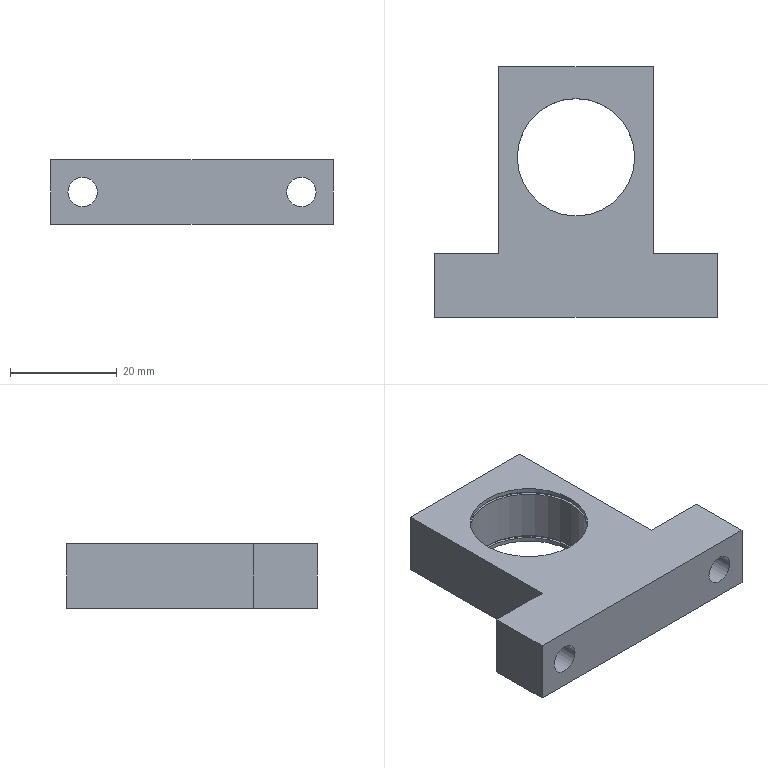Part | SolidWorks | features ICE 4, Extrusion 1 | 1 solid | 34 faces | box 53 x 47 x 12 mm | volume 14009 mm3 | cylinder 18 | plane 16 | commonest cylinder face diameters 22 x6 5.5 x4 10 x4 23 x4
STEP:
#1=CARTESIAN_POINT('',(21.73,13.962,1.25));
#2=VERTEX_POINT('',#1);
#3=CARTESIAN_POINT('',(-1.27,13.962,1.25));
#4=VERTEX_POINT('',#3);
#5=CARTESIAN_POINT('',(10.23,13.962,1.25));
#6=DIRECTION('',(0.,0.,-1.));
#7=DIRECTION('',(-1.,0.,0.));
#8=AXIS2_PLACEMENT_3D('',#5,#6,#7);
#9=CIRCLE('',#8,11.5);
#10=EDGE_CURVE('',#2,#4,#9,.T.);
#11=ORIENTED_EDGE('',*,*,#10,.F.);
#12=CARTESIAN_POINT('',(21.73,13.962,0.75));
#13=VERTEX_POINT('',#12);
#14=CARTESIAN_POINT('',(21.73,13.962,1.25));
#15=DIRECTION('',(0.,0.,-1.));
#16=VECTOR('',#15,1000.);
#17=LINE('',#14,#16);
#18=EDGE_CURVE('',#2,#13,#17,.T.);
#19=ORIENTED_EDGE('',*,*,#18,.T.);
#20=CARTESIAN_POINT('',(-1.27,13.962,0.75));
#21=VERTEX_POINT('',#20);
#22=CARTESIAN_POINT('',(10.23,13.962,0.75));
#23=DIRECTION('',(0.,0.,-1.));
#24=DIRECTION('',(-1.,0.,0.));
#25=AXIS2_PLACEMENT_3D('',#22,#23,#24);
#26=CIRCLE('',#25,11.5);
#27=EDGE_CURVE('',#13,#21,#26,.T.);
#28=ORIENTED_EDGE('',*,*,#27,.T.);
#29=CARTESIAN_POINT('',(-1.27,13.962,1.25));
#30=DIRECTION('',(0.,0.,-1.));
#31=VECTOR('',#30,1000.);
#32=LINE('',#29,#31);
#33=EDGE_CURVE('',#4,#21,#32,.T.);
#34=ORIENTED_EDGE('',*,*,#33,.F.);
#35=EDGE_LOOP('',(#11,#19,#28,#34));
#36=FACE_OUTER_BOUND('',#35,.T.);
#37=CARTESIAN_POINT('',(10.23,13.962,1.25));
#38=DIRECTION('',(0.,0.,-1.));
#39=DIRECTION('',(-1.,0.,0.));
#40=AXIS2_PLACEMENT_3D('',#37,#38,#39);
#41=CYLINDRICAL_SURFACE('',#40,11.5);
#42=ADVANCED_FACE('',(#36),#41,.F.);
#43=CARTESIAN_POINT('',(-1.27,13.962,10.75));
#44=VERTEX_POINT('',#43);
#45=CARTESIAN_POINT('',(21.73,13.962,10.75));
#46=VERTEX_POINT('',#45);
#47=CARTESIAN_POINT('',(10.23,13.962,10.75));
#48=DIRECTION('',(0.,0.,1.));
#49=DIRECTION('',(1.,0.,0.));
#50=AXIS2_PLACEMENT_3D('',#47,#48,#49);
#51=CIRCLE('',#50,11.5);
#52=EDGE_CURVE('',#44,#46,#51,.T.);
#53=ORIENTED_EDGE('',*,*,#52,.F.);
#54=CARTESIAN_POINT('',(-1.27,13.962,11.25));
#55=VERTEX_POINT('',#54);
#56=CARTESIAN_POINT('',(-1.27,13.962,10.75));
#57=DIRECTION('',(0.,0.,1.));
#58=VECTOR('',#57,1000.);
#59=LINE('',#56,#58);
#60=EDGE_CURVE('',#44,#55,#59,.T.);
#61=ORIENTED_EDGE('',*,*,#60,.T.);
#62=CARTESIAN_POINT('',(21.73,13.962,11.25));
#63=VERTEX_POINT('',#62);
#64=CARTESIAN_POINT('',(10.23,13.962,11.25));
#65=DIRECTION('',(0.,0.,1.));
#66=DIRECTION('',(1.,0.,0.));
#67=AXIS2_PLACEMENT_3D('',#64,#65,#66);
#68=CIRCLE('',#67,11.5);
#69=EDGE_CURVE('',#55,#63,#68,.T.);
#70=ORIENTED_EDGE('',*,*,#69,.T.);
#71=CARTESIAN_POINT('',(21.73,13.962,10.75));
#72=DIRECTION('',(0.,0.,1.));
#73=VECTOR('',#72,1000.);
#74=LINE('',#71,#73);
#75=EDGE_CURVE('',#46,#63,#74,.T.);
#76=ORIENTED_EDGE('',*,*,#75,.F.);
#77=EDGE_LOOP('',(#53,#61,#70,#76));
#78=FACE_OUTER_BOUND('',#77,.T.);
#79=CARTESIAN_POINT('',(10.23,13.962,10.75));
#80=DIRECTION('',(0.,0.,1.));
#81=DIRECTION('',(1.,0.,0.));
#82=AXIS2_PLACEMENT_3D('',#79,#80,#81);
#83=CYLINDRICAL_SURFACE('',#82,11.5);
#84=ADVANCED_FACE('',(#78),#83,.F.);
#85=CARTESIAN_POINT('',(-5.27,-9.838,6.));
#86=VERTEX_POINT('',#85);
#87=CARTESIAN_POINT('',(-15.27,-9.838,6.));
#88=VERTEX_POINT('',#87);
#89=CARTESIAN_POINT('',(-10.27,-9.838,6.));
#90=DIRECTION('',(0.,1.,0.));
#91=DIRECTION('',(-1.,0.,0.));
#92=AXIS2_PLACEMENT_3D('',#89,#90,#91);
#93=CIRCLE('',#92,5.);
#94=EDGE_CURVE('',#86,#88,#93,.T.);
#95=ORIENTED_EDGE('',*,*,#94,.F.);
#96=CARTESIAN_POINT('',(-5.27,-4.038,6.));
#97=VERTEX_POINT('',#96);
#98=CARTESIAN_POINT('',(-5.27,-9.838,6.));
#99=DIRECTION('',(0.,1.,0.));
#100=VECTOR('',#99,1000.);
#101=LINE('',#98,#100);
#102=EDGE_CURVE('',#86,#97,#101,.T.);
#103=ORIENTED_EDGE('',*,*,#102,.T.);
#104=CARTESIAN_POINT('',(-15.27,-4.038,6.));
#105=VERTEX_POINT('',#104);
#106=CARTESIAN_POINT('',(-10.27,-4.038,6.));
#107=DIRECTION('',(0.,1.,0.));
#108=DIRECTION('',(-1.,0.,0.));
#109=AXIS2_PLACEMENT_3D('',#106,#107,#108);
#110=CIRCLE('',#109,5.);
#111=EDGE_CURVE('',#97,#105,#110,.T.);
#112=ORIENTED_EDGE('',*,*,#111,.T.);
#113=CARTESIAN_POINT('',(-15.27,-9.838,6.));
#114=DIRECTION('',(0.,1.,0.));
#115=VECTOR('',#114,1000.);
#116=LINE('',#113,#115);
#117=EDGE_CURVE('',#88,#105,#116,.T.);
#118=ORIENTED_EDGE('',*,*,#117,.F.);
#119=EDGE_LOOP('',(#95,#103,#112,#118));
#120=FACE_OUTER_BOUND('',#119,.T.);
#121=CARTESIAN_POINT('',(-10.27,-9.838,6.));
#122=DIRECTION('',(0.,1.,0.));
#123=DIRECTION('',(-1.,0.,0.));
#124=AXIS2_PLACEMENT_3D('',#121,#122,#123);
#125=CYLINDRICAL_SURFACE('',#124,5.);
#126=ADVANCED_FACE('',(#120),#125,.F.);
#127=CARTESIAN_POINT('',(35.73,-9.838,6.));
#128=VERTEX_POINT('',#127);
#129=CARTESIAN_POINT('',(25.73,-9.838,6.));
#130=VERTEX_POINT('',#129);
#131=CARTESIAN_POINT('',(30.73,-9.838,6.));
#132=DIRECTION('',(0.,1.,0.));
#133=DIRECTION('',(-1.,0.,0.));
#134=AXIS2_PLACEMENT_3D('',#131,#132,#133);
#135=CIRCLE('',#134,5.);
#136=EDGE_CURVE('',#128,#130,#135,.T.);
#137=ORIENTED_EDGE('',*,*,#136,.F.);
#138=CARTESIAN_POINT('',(35.73,-4.038,6.));
#139=VERTEX_POINT('',#138);
#140=CARTESIAN_POINT('',(35.73,-9.838,6.));
#141=DIRECTION('',(0.,1.,0.));
#142=VECTOR('',#141,1000.);
#143=LINE('',#140,#142);
#144=EDGE_CURVE('',#128,#139,#143,.T.);
#145=ORIENTED_EDGE('',*,*,#144,.T.);
#146=CARTESIAN_POINT('',(25.73,-4.038,6.));
#147=VERTEX_POINT('',#146);
#148=CARTESIAN_POINT('',(30.73,-4.038,6.));
#149=DIRECTION('',(0.,1.,0.));
#150=DIRECTION('',(-1.,0.,0.));
#151=AXIS2_PLACEMENT_3D('',#148,#149,#150);
#152=CIRCLE('',#151,5.);
#153=EDGE_CURVE('',#139,#147,#152,.T.);
#154=ORIENTED_EDGE('',*,*,#153,.T.);
#155=CARTESIAN_POINT('',(25.73,-9.838,6.));
#156=DIRECTION('',(0.,1.,0.));
#157=VECTOR('',#156,1000.);
#158=LINE('',#155,#157);
#159=EDGE_CURVE('',#130,#147,#158,.T.);
#160=ORIENTED_EDGE('',*,*,#159,.F.);
#161=EDGE_LOOP('',(#137,#145,#154,#160));
#162=FACE_OUTER_BOUND('',#161,.T.);
#163=CARTESIAN_POINT('',(30.73,-9.838,6.));
#164=DIRECTION('',(0.,1.,0.));
#165=DIRECTION('',(-1.,0.,0.));
#166=AXIS2_PLACEMENT_3D('',#163,#164,#165);
#167=CYLINDRICAL_SURFACE('',#166,5.);
#168=ADVANCED_FACE('',(#162),#167,.F.);
#169=CARTESIAN_POINT('',(-0.7697,13.962,12.));
#170=VERTEX_POINT('',#169);
#171=CARTESIAN_POINT('',(21.23,13.962,12.));
#172=VERTEX_POINT('',#171);
#173=CARTESIAN_POINT('',(10.23,13.962,12.));
#174=DIRECTION('',(0.,0.,1.));
#175=DIRECTION('',(1.,0.,0.));
#176=AXIS2_PLACEMENT_3D('',#173,#174,#175);
#177=CIRCLE('',#176,11.);
#178=EDGE_CURVE('',#170,#172,#177,.T.);
#179=ORIENTED_EDGE('',*,*,#178,.T.);
#180=CARTESIAN_POINT('',(21.23,13.962,11.25));
#181=VERTEX_POINT('',#180);
#182=CARTESIAN_POINT('',(21.23,13.962,12.));
#183=DIRECTION('',(0.,0.,-1.));
#184=VECTOR('',#183,1000.);
#185=LINE('',#182,#184);
#186=EDGE_CURVE('',#172,#181,#185,.T.);
#187=ORIENTED_EDGE('',*,*,#186,.T.);
#188=CARTESIAN_POINT('',(-0.7697,13.962,11.25));
#189=VERTEX_POINT('',#188);
#190=CARTESIAN_POINT('',(10.23,13.962,11.25));
#191=DIRECTION('',(0.,0.,1.));
#192=DIRECTION('',(1.,0.,0.));
#193=AXIS2_PLACEMENT_3D('',#190,#191,#192);
#194=CIRCLE('',#193,11.);
#195=EDGE_CURVE('',#189,#181,#194,.T.);
#196=ORIENTED_EDGE('',*,*,#195,.F.);
#197=CARTESIAN_POINT('',(-0.7697,13.962,12.));
#198=DIRECTION('',(0.,0.,-1.));
#199=VECTOR('',#198,1000.);
#200=LINE('',#197,#199);
#201=EDGE_CURVE('',#170,#189,#200,.T.);
#202=ORIENTED_EDGE('',*,*,#201,.F.);
#203=EDGE_LOOP('',(#179,#187,#196,#202));
#204=FACE_OUTER_BOUND('',#203,.T.);
#205=CARTESIAN_POINT('',(10.23,13.962,12.));
#206=DIRECTION('',(0.,0.,-1.));
#207=DIRECTION('',(-1.,0.,0.));
#208=AXIS2_PLACEMENT_3D('',#205,#206,#207);
#209=CYLINDRICAL_SURFACE('',#208,11.);
#210=ADVANCED_FACE('',(#204),#209,.F.);
#211=CARTESIAN_POINT('',(33.48,-16.038,6.));
#212=VERTEX_POINT('',#211);
#213=CARTESIAN_POINT('',(27.98,-16.038,6.));
#214=VERTEX_POINT('',#213);
#215=CARTESIAN_POINT('',(30.73,-16.038,6.));
#216=DIRECTION('',(0.,1.,0.));
#217=DIRECTION('',(-1.,0.,0.));
#218=AXIS2_PLACEMENT_3D('',#215,#216,#217);
#219=CIRCLE('',#218,2.75);
#220=EDGE_CURVE('',#212,#214,#219,.T.);
#221=ORIENTED_EDGE('',*,*,#220,.F.);
#222=CARTESIAN_POINT('',(33.48,-9.838,6.));
#223=VERTEX_POINT('',#222);
#224=CARTESIAN_POINT('',(33.48,-16.038,6.));
#225=DIRECTION('',(0.,1.,0.));
#226=VECTOR('',#225,1000.);
#227=LINE('',#224,#226);
#228=EDGE_CURVE('',#212,#223,#227,.T.);
#229=ORIENTED_EDGE('',*,*,#228,.T.);
#230=CARTESIAN_POINT('',(27.98,-9.838,6.));
#231=VERTEX_POINT('',#230);
#232=CARTESIAN_POINT('',(30.73,-9.838,6.));
#233=DIRECTION('',(0.,-1.,0.));
#234=DIRECTION('',(-1.,0.,0.));
#235=AXIS2_PLACEMENT_3D('',#232,#233,#234);
#236=CIRCLE('',#235,2.75);
#237=EDGE_CURVE('',#231,#223,#236,.T.);
#238=ORIENTED_EDGE('',*,*,#237,.F.);
#239=CARTESIAN_POINT('',(27.98,-16.038,6.));
#240=DIRECTION('',(0.,1.,0.));
#241=VECTOR('',#240,1000.);
#242=LINE('',#239,#241);
#243=EDGE_CURVE('',#214,#231,#242,.T.);
#244=ORIENTED_EDGE('',*,*,#243,.F.);
#245=EDGE_LOOP('',(#221,#229,#238,#244));
#246=FACE_OUTER_BOUND('',#245,.T.);
#247=CARTESIAN_POINT('',(30.73,-16.038,6.));
#248=DIRECTION('',(0.,1.,0.));
#249=DIRECTION('',(-1.,0.,0.));
#250=AXIS2_PLACEMENT_3D('',#247,#248,#249);
#251=CYLINDRICAL_SURFACE('',#250,2.75);
#252=ADVANCED_FACE('',(#246),#251,.F.);
#253=CARTESIAN_POINT('',(-7.52,-16.038,6.));
#254=VERTEX_POINT('',#253);
#255=CARTESIAN_POINT('',(-13.02,-16.038,6.));
#256=VERTEX_POINT('',#255);
#257=CARTESIAN_POINT('',(-10.27,-16.038,6.));
#258=DIRECTION('',(0.,1.,0.));
#259=DIRECTION('',(-1.,0.,0.));
#260=AXIS2_PLACEMENT_3D('',#257,#258,#259);
#261=CIRCLE('',#260,2.75);
#262=EDGE_CURVE('',#254,#256,#261,.T.);
#263=ORIENTED_EDGE('',*,*,#262,.F.);
#264=CARTESIAN_POINT('',(-7.52,-9.838,6.));
#265=VERTEX_POINT('',#264);
#266=CARTESIAN_POINT('',(-7.52,-16.038,6.));
#267=DIRECTION('',(0.,1.,0.));
#268=VECTOR('',#267,1000.);
#269=LINE('',#266,#268);
#270=EDGE_CURVE('',#254,#265,#269,.T.);
#271=ORIENTED_EDGE('',*,*,#270,.T.);
#272=CARTESIAN_POINT('',(-13.02,-9.838,6.));
#273=VERTEX_POINT('',#272);
#274=CARTESIAN_POINT('',(-10.27,-9.838,6.));
#275=DIRECTION('',(0.,-1.,0.));
#276=DIRECTION('',(-1.,0.,0.));
#277=AXIS2_PLACEMENT_3D('',#274,#275,#276);
#278=CIRCLE('',#277,2.75);
#279=EDGE_CURVE('',#273,#265,#278,.T.);
#280=ORIENTED_EDGE('',*,*,#279,.F.);
#281=CARTESIAN_POINT('',(-13.02,-16.038,6.));
#282=DIRECTION('',(0.,1.,0.));
#283=VECTOR('',#282,1000.);
#284=LINE('',#281,#283);
#285=EDGE_CURVE('',#256,#273,#284,.T.);
#286=ORIENTED_EDGE('',*,*,#285,.F.);
#287=EDGE_LOOP('',(#263,#271,#280,#286));
#288=FACE_OUTER_BOUND('',#287,.T.);
#289=CARTESIAN_POINT('',(-10.27,-16.038,6.));
#290=DIRECTION('',(0.,1.,0.));
#291=DIRECTION('',(-1.,0.,0.));
#292=AXIS2_PLACEMENT_3D('',#289,#290,#291);
#293=CYLINDRICAL_SURFACE('',#292,2.75);
#294=ADVANCED_FACE('',(#288),#293,.F.);
#295=CARTESIAN_POINT('',(21.23,13.962,0.75));
#296=VERTEX_POINT('',#295);
#297=CARTESIAN_POINT('',(-0.7697,13.962,0.75));
#298=VERTEX_POINT('',#297);
#299=CARTESIAN_POINT('',(10.23,13.962,0.75));
#300=DIRECTION('',(0.,0.,-1.));
#301=DIRECTION('',(-1.,0.,0.));
#302=AXIS2_PLACEMENT_3D('',#299,#300,#301);
#303=CIRCLE('',#302,11.);
#304=EDGE_CURVE('',#296,#298,#303,.T.);
#305=ORIENTED_EDGE('',*,*,#304,.F.);
#306=CARTESIAN_POINT('',(21.23,13.962,0.));
#307=VERTEX_POINT('',#306);
#308=CARTESIAN_POINT('',(21.23,13.962,12.));
#309=DIRECTION('',(0.,0.,-1.));
#310=VECTOR('',#309,1000.);
#311=LINE('',#308,#310);
#312=EDGE_CURVE('',#296,#307,#311,.T.);
#313=ORIENTED_EDGE('',*,*,#312,.T.);
#314=CARTESIAN_POINT('',(-0.7697,13.962,0.));
#315=VERTEX_POINT('',#314);
#316=CARTESIAN_POINT('',(10.23,13.962,0.));
#317=DIRECTION('',(0.,0.,1.));
#318=DIRECTION('',(1.,0.,0.));
#319=AXIS2_PLACEMENT_3D('',#316,#317,#318);
#320=CIRCLE('',#319,11.);
#321=EDGE_CURVE('',#315,#307,#320,.T.);
#322=ORIENTED_EDGE('',*,*,#321,.F.);
#323=CARTESIAN_POINT('',(-0.7697,13.962,12.));
#324=DIRECTION('',(0.,0.,-1.));
#325=VECTOR('',#324,1000.);
#326=LINE('',#323,#325);
#327=EDGE_CURVE('',#298,#315,#326,.T.);
#328=ORIENTED_EDGE('',*,*,#327,.F.);
#329=EDGE_LOOP('',(#305,#313,#322,#328));
#330=FACE_OUTER_BOUND('',#329,.T.);
#331=CARTESIAN_POINT('',(10.23,13.962,12.));
#332=DIRECTION('',(0.,0.,-1.));
#333=DIRECTION('',(-1.,0.,0.));
#334=AXIS2_PLACEMENT_3D('',#331,#332,#333);
#335=CYLINDRICAL_SURFACE('',#334,11.);
#336=ADVANCED_FACE('',(#330),#335,.F.);
#337=CARTESIAN_POINT('',(-0.7697,13.962,10.75));
#338=VERTEX_POINT('',#337);
#339=CARTESIAN_POINT('',(21.23,13.962,10.75));
#340=VERTEX_POINT('',#339);
#341=CARTESIAN_POINT('',(10.23,13.962,10.75));
#342=DIRECTION('',(0.,0.,1.));
#343=DIRECTION('',(1.,0.,0.));
#344=AXIS2_PLACEMENT_3D('',#341,#342,#343);
#345=CIRCLE('',#344,11.);
#346=EDGE_CURVE('',#338,#340,#345,.T.);
#347=ORIENTED_EDGE('',*,*,#346,.T.);
#348=CARTESIAN_POINT('',(21.23,13.962,1.25));
#349=VERTEX_POINT('',#348);
#350=CARTESIAN_POINT('',(21.23,13.962,12.));
#351=DIRECTION('',(0.,0.,-1.));
#352=VECTOR('',#351,1000.);
#353=LINE('',#350,#352);
#354=EDGE_CURVE('',#340,#349,#353,.T.);
#355=ORIENTED_EDGE('',*,*,#354,.T.);
#356=CARTESIAN_POINT('',(-0.7697,13.962,1.25));
#357=VERTEX_POINT('',#356);
#358=CARTESIAN_POINT('',(10.23,13.962,1.25));
#359=DIRECTION('',(0.,0.,-1.));
#360=DIRECTION('',(-1.,0.,0.));
#361=AXIS2_PLACEMENT_3D('',#358,#359,#360);
#362=CIRCLE('',#361,11.);
#363=EDGE_CURVE('',#349,#357,#362,.T.);
#364=ORIENTED_EDGE('',*,*,#363,.T.);
#365=CARTESIAN_POINT('',(-0.7697,13.962,12.));
#366=DIRECTION('',(0.,0.,-1.));
#367=VECTOR('',#366,1000.);
#368=LINE('',#365,#367);
#369=EDGE_CURVE('',#338,#357,#368,.T.);
#370=ORIENTED_EDGE('',*,*,#369,.F.);
#371=EDGE_LOOP('',(#347,#355,#364,#370));
#372=FACE_OUTER_BOUND('',#371,.T.);
#373=CARTESIAN_POINT('',(10.23,13.962,12.));
#374=DIRECTION('',(0.,0.,-1.));
#375=DIRECTION('',(-1.,0.,0.));
#376=AXIS2_PLACEMENT_3D('',#373,#374,#375);
#377=CYLINDRICAL_SURFACE('',#376,11.);
#378=ADVANCED_FACE('',(#372),#377,.F.);
#379=ORIENTED_EDGE('',*,*,#354,.F.);
#380=CARTESIAN_POINT('',(10.23,13.962,10.75));
#381=DIRECTION('',(0.,0.,1.));
#382=DIRECTION('',(1.,0.,0.));
#383=AXIS2_PLACEMENT_3D('',#380,#381,#382);
#384=CIRCLE('',#383,11.);
#385=EDGE_CURVE('',#340,#338,#384,.T.);
#386=ORIENTED_EDGE('',*,*,#385,.T.);
#387=ORIENTED_EDGE('',*,*,#369,.T.);
#388=CARTESIAN_POINT('',(10.23,13.962,1.25));
#389=DIRECTION('',(0.,0.,-1.));
#390=DIRECTION('',(-1.,0.,0.));
#391=AXIS2_PLACEMENT_3D('',#388,#389,#390);
#392=CIRCLE('',#391,11.);
#393=EDGE_CURVE('',#357,#349,#392,.T.);
#394=ORIENTED_EDGE('',*,*,#393,.T.);
#395=EDGE_LOOP('',(#379,#386,#387,#394));
#396=FACE_OUTER_BOUND('',#395,.T.);
#397=CARTESIAN_POINT('',(10.23,13.962,12.));
#398=DIRECTION('',(0.,0.,-1.));
#399=DIRECTION('',(-1.,0.,0.));
#400=AXIS2_PLACEMENT_3D('',#397,#398,#399);
#401=CYLINDRICAL_SURFACE('',#400,11.);
#402=ADVANCED_FACE('',(#396),#401,.F.);
#403=ORIENTED_EDGE('',*,*,#312,.F.);
#404=CARTESIAN_POINT('',(10.23,13.962,0.75));
#405=DIRECTION('',(0.,0.,-1.));
#406=DIRECTION('',(-1.,0.,0.));
#407=AXIS2_PLACEMENT_3D('',#404,#405,#406);
#408=CIRCLE('',#407,11.);
#409=EDGE_CURVE('',#298,#296,#408,.T.);
#410=ORIENTED_EDGE('',*,*,#409,.F.);
#411=ORIENTED_EDGE('',*,*,#327,.T.);
#412=CARTESIAN_POINT('',(10.23,13.962,0.));
#413=DIRECTION('',(0.,0.,1.));
#414=DIRECTION('',(1.,0.,0.));
#415=AXIS2_PLACEMENT_3D('',#412,#413,#414);
#416=CIRCLE('',#415,11.);
#417=EDGE_CURVE('',#307,#315,#416,.T.);
#418=ORIENTED_EDGE('',*,*,#417,.F.);
#419=EDGE_LOOP('',(#403,#410,#411,#418));
#420=FACE_OUTER_BOUND('',#419,.T.);
#421=CARTESIAN_POINT('',(10.23,13.962,12.));
#422=DIRECTION('',(0.,0.,-1.));
#423=DIRECTION('',(-1.,0.,0.));
#424=AXIS2_PLACEMENT_3D('',#421,#422,#423);
#425=CYLINDRICAL_SURFACE('',#424,11.);
#426=ADVANCED_FACE('',(#420),#425,.F.);
#427=ORIENTED_EDGE('',*,*,#270,.F.);
#428=CARTESIAN_POINT('',(-10.27,-16.038,6.));
#429=DIRECTION('',(0.,1.,0.));
#430=DIRECTION('',(-1.,0.,0.));
#431=AXIS2_PLACEMENT_3D('',#428,#429,#430);
#432=CIRCLE('',#431,2.75);
#433=EDGE_CURVE('',#256,#254,#432,.T.);
#434=ORIENTED_EDGE('',*,*,#433,.F.);
#435=ORIENTED_EDGE('',*,*,#285,.T.);
#436=CARTESIAN_POINT('',(-10.27,-9.838,6.));
#437=DIRECTION('',(0.,-1.,0.));
#438=DIRECTION('',(-1.,0.,0.));
#439=AXIS2_PLACEMENT_3D('',#436,#437,#438);
#440=CIRCLE('',#439,2.75);
#441=EDGE_CURVE('',#265,#273,#440,.T.);
#442=ORIENTED_EDGE('',*,*,#441,.F.);
#443=EDGE_LOOP('',(#427,#434,#435,#442));
#444=FACE_OUTER_BOUND('',#443,.T.);
#445=CARTESIAN_POINT('',(-10.27,-16.038,6.));
#446=DIRECTION('',(0.,1.,0.));
#447=DIRECTION('',(-1.,0.,0.));
#448=AXIS2_PLACEMENT_3D('',#445,#446,#447);
#449=CYLINDRICAL_SURFACE('',#448,2.75);
#450=ADVANCED_FACE('',(#444),#449,.F.);
#451=ORIENTED_EDGE('',*,*,#228,.F.);
#452=CARTESIAN_POINT('',(30.73,-16.038,6.));
#453=DIRECTION('',(0.,1.,0.));
#454=DIRECTION('',(-1.,0.,0.));
#455=AXIS2_PLACEMENT_3D('',#452,#453,#454);
#456=CIRCLE('',#455,2.75);
#457=EDGE_CURVE('',#214,#212,#456,.T.);
#458=ORIENTED_EDGE('',*,*,#457,.F.);
#459=ORIENTED_EDGE('',*,*,#243,.T.);
#460=CARTESIAN_POINT('',(30.73,-9.838,6.));
#461=DIRECTION('',(0.,-1.,0.));
#462=DIRECTION('',(-1.,0.,0.));
#463=AXIS2_PLACEMENT_3D('',#460,#461,#462);
#464=CIRCLE('',#463,2.75);
#465=EDGE_CURVE('',#223,#231,#464,.T.);
#466=ORIENTED_EDGE('',*,*,#465,.F.);
#467=EDGE_LOOP('',(#451,#458,#459,#466));
#468=FACE_OUTER_BOUND('',#467,.T.);
#469=CARTESIAN_POINT('',(30.73,-16.038,6.));
#470=DIRECTION('',(0.,1.,0.));
#471=DIRECTION('',(-1.,0.,0.));
#472=AXIS2_PLACEMENT_3D('',#469,#470,#471);
#473=CYLINDRICAL_SURFACE('',#472,2.75);
#474=ADVANCED_FACE('',(#468),#473,.F.);
#475=CARTESIAN_POINT('',(-16.27,-4.038,12.));
#476=VERTEX_POINT('',#475);
#477=CARTESIAN_POINT('',(-16.27,-16.038,12.));
#478=VERTEX_POINT('',#477);
#479=CARTESIAN_POINT('',(-16.27,-4.038,12.));
#480=DIRECTION('',(0.,-1.,0.));
#481=VECTOR('',#480,1000.);
#482=LINE('',#479,#481);
#483=EDGE_CURVE('',#476,#478,#482,.T.);
#484=ORIENTED_EDGE('',*,*,#483,.T.);
#485=CARTESIAN_POINT('',(36.73,-16.038,12.));
#486=VERTEX_POINT('',#485);
#487=CARTESIAN_POINT('',(-16.27,-16.038,12.));
#488=DIRECTION('',(1.,0.,0.));
#489=VECTOR('',#488,1000.);
#490=LINE('',#487,#489);
#491=EDGE_CURVE('',#478,#486,#490,.T.);
#492=ORIENTED_EDGE('',*,*,#491,.T.);
#493=CARTESIAN_POINT('',(36.73,-4.038,12.));
#494=VERTEX_POINT('',#493);
#495=CARTESIAN_POINT('',(36.73,-16.038,12.));
#496=DIRECTION('',(0.,1.,0.));
#497=VECTOR('',#496,1000.);
#498=LINE('',#495,#497);
#499=EDGE_CURVE('',#486,#494,#498,.T.);
#500=ORIENTED_EDGE('',*,*,#499,.T.);
#501=CARTESIAN_POINT('',(24.73,-4.038,12.));
#502=VERTEX_POINT('',#501);
#503=CARTESIAN_POINT('',(36.73,-4.038,12.));
#504=DIRECTION('',(-1.,0.,0.));
#505=VECTOR('',#504,1000.);
#506=LINE('',#503,#505);
#507=EDGE_CURVE('',#494,#502,#506,.T.);
#508=ORIENTED_EDGE('',*,*,#507,.T.);
#509=CARTESIAN_POINT('',(24.73,30.962,12.));
#510=VERTEX_POINT('',#509);
#511=CARTESIAN_POINT('',(24.73,-4.038,12.));
#512=DIRECTION('',(0.,1.,0.));
#513=VECTOR('',#512,1000.);
#514=LINE('',#511,#513);
#515=EDGE_CURVE('',#502,#510,#514,.T.);
#516=ORIENTED_EDGE('',*,*,#515,.T.);
#517=CARTESIAN_POINT('',(-4.27,30.962,12.));
#518=VERTEX_POINT('',#517);
#519=CARTESIAN_POINT('',(24.73,30.962,12.));
#520=DIRECTION('',(-1.,0.,0.));
#521=VECTOR('',#520,1000.);
#522=LINE('',#519,#521);
#523=EDGE_CURVE('',#510,#518,#522,.T.);
#524=ORIENTED_EDGE('',*,*,#523,.T.);
#525=CARTESIAN_POINT('',(-4.27,-4.038,12.));
#526=VERTEX_POINT('',#525);
#527=CARTESIAN_POINT('',(-4.27,30.962,12.));
#528=DIRECTION('',(0.,-1.,0.));
#529=VECTOR('',#528,1000.);
#530=LINE('',#527,#529);
#531=EDGE_CURVE('',#518,#526,#530,.T.);
#532=ORIENTED_EDGE('',*,*,#531,.T.);
#533=CARTESIAN_POINT('',(-4.27,-4.038,12.));
#534=DIRECTION('',(-1.,0.,0.));
#535=VECTOR('',#534,1000.);
#536=LINE('',#533,#535);
#537=EDGE_CURVE('',#526,#476,#536,.T.);
#538=ORIENTED_EDGE('',*,*,#537,.T.);
#539=EDGE_LOOP('',(#484,#492,#500,#508,#516,#524,#532,#538));
#540=FACE_OUTER_BOUND('',#539,.T.);
#541=ORIENTED_EDGE('',*,*,#178,.F.);
#542=CARTESIAN_POINT('',(10.23,13.962,12.));
#543=DIRECTION('',(0.,0.,1.));
#544=DIRECTION('',(1.,0.,0.));
#545=AXIS2_PLACEMENT_3D('',#542,#543,#544);
#546=CIRCLE('',#545,11.);
#547=EDGE_CURVE('',#172,#170,#546,.T.);
#548=ORIENTED_EDGE('',*,*,#547,.F.);
#549=EDGE_LOOP('',(#541,#548));
#550=FACE_BOUND('',#549,.T.);
#551=CARTESIAN_POINT('',(0.,0.,12.));
#552=DIRECTION('',(0.,0.,1.));
#553=DIRECTION('',(1.,0.,0.));
#554=AXIS2_PLACEMENT_3D('',#551,#552,#553);
#555=PLANE('',#554);
#556=ADVANCED_FACE('',(#540,#550),#555,.T.);
#557=CARTESIAN_POINT('',(-16.27,-4.038,0.));
#558=VERTEX_POINT('',#557);
#559=CARTESIAN_POINT('',(-16.27,-16.038,0.));
#560=VERTEX_POINT('',#559);
#561=CARTESIAN_POINT('',(-16.27,-4.038,0.));
#562=DIRECTION('',(0.,-1.,0.));
#563=VECTOR('',#562,1000.);
#564=LINE('',#561,#563);
#565=EDGE_CURVE('',#558,#560,#564,.T.);
#566=ORIENTED_EDGE('',*,*,#565,.F.);
#567=CARTESIAN_POINT('',(-4.27,-4.038,0.));
#568=VERTEX_POINT('',#567);
#569=CARTESIAN_POINT('',(-4.27,-4.038,0.));
#570=DIRECTION('',(-1.,0.,0.));
#571=VECTOR('',#570,1000.);
#572=LINE('',#569,#571);
#573=EDGE_CURVE('',#568,#558,#572,.T.);
#574=ORIENTED_EDGE('',*,*,#573,.F.);
#575=CARTESIAN_POINT('',(-4.27,30.962,0.));
#576=VERTEX_POINT('',#575);
#577=CARTESIAN_POINT('',(-4.27,30.962,0.));
#578=DIRECTION('',(0.,-1.,0.));
#579=VECTOR('',#578,1000.);
#580=LINE('',#577,#579);
#581=EDGE_CURVE('',#576,#568,#580,.T.);
#582=ORIENTED_EDGE('',*,*,#581,.F.);
#583=CARTESIAN_POINT('',(24.73,30.962,0.));
#584=VERTEX_POINT('',#583);
#585=CARTESIAN_POINT('',(24.73,30.962,0.));
#586=DIRECTION('',(-1.,0.,0.));
#587=VECTOR('',#586,1000.);
#588=LINE('',#585,#587);
#589=EDGE_CURVE('',#584,#576,#588,.T.);
#590=ORIENTED_EDGE('',*,*,#589,.F.);
#591=CARTESIAN_POINT('',(24.73,-4.038,0.));
#592=VERTEX_POINT('',#591);
#593=CARTESIAN_POINT('',(24.73,-4.038,0.));
#594=DIRECTION('',(0.,1.,0.));
#595=VECTOR('',#594,1000.);
#596=LINE('',#593,#595);
#597=EDGE_CURVE('',#592,#584,#596,.T.);
#598=ORIENTED_EDGE('',*,*,#597,.F.);
#599=CARTESIAN_POINT('',(36.73,-4.038,0.));
#600=VERTEX_POINT('',#599);
#601=CARTESIAN_POINT('',(36.73,-4.038,0.));
#602=DIRECTION('',(-1.,0.,0.));
#603=VECTOR('',#602,1000.);
#604=LINE('',#601,#603);
#605=EDGE_CURVE('',#600,#592,#604,.T.);
#606=ORIENTED_EDGE('',*,*,#605,.F.);
#607=CARTESIAN_POINT('',(36.73,-16.038,0.));
#608=VERTEX_POINT('',#607);
#609=CARTESIAN_POINT('',(36.73,-16.038,0.));
#610=DIRECTION('',(0.,1.,0.));
#611=VECTOR('',#610,1000.);
#612=LINE('',#609,#611);
#613=EDGE_CURVE('',#608,#600,#612,.T.);
#614=ORIENTED_EDGE('',*,*,#613,.F.);
#615=CARTESIAN_POINT('',(-16.27,-16.038,0.));
#616=DIRECTION('',(1.,0.,0.));
#617=VECTOR('',#616,1000.);
#618=LINE('',#615,#617);
#619=EDGE_CURVE('',#560,#608,#618,.T.);
#620=ORIENTED_EDGE('',*,*,#619,.F.);
#621=EDGE_LOOP('',(#566,#574,#582,#590,#598,#606,#614,#620));
#622=FACE_OUTER_BOUND('',#621,.T.);
#623=ORIENTED_EDGE('',*,*,#321,.T.);
#624=ORIENTED_EDGE('',*,*,#417,.T.);
#625=EDGE_LOOP('',(#623,#624));
#626=FACE_BOUND('',#625,.T.);
#627=CARTESIAN_POINT('',(0.,0.,0.));
#628=DIRECTION('',(0.,0.,1.));
#629=DIRECTION('',(1.,0.,0.));
#630=AXIS2_PLACEMENT_3D('',#627,#628,#629);
#631=PLANE('',#630);
#632=ADVANCED_FACE('',(#622,#626),#631,.F.);
#633=ORIENTED_EDGE('',*,*,#565,.T.);
#634=CARTESIAN_POINT('',(-16.27,-16.038,12.));
#635=DIRECTION('',(0.,0.,-1.));
#636=VECTOR('',#635,1000.);
#637=LINE('',#634,#636);
#638=EDGE_CURVE('',#478,#560,#637,.T.);
#639=ORIENTED_EDGE('',*,*,#638,.F.);
#640=ORIENTED_EDGE('',*,*,#483,.F.);
#641=CARTESIAN_POINT('',(-16.27,-4.038,12.));
#642=DIRECTION('',(0.,0.,-1.));
#643=VECTOR('',#642,1000.);
#644=LINE('',#641,#643);
#645=EDGE_CURVE('',#476,#558,#644,.T.);
#646=ORIENTED_EDGE('',*,*,#645,.T.);
#647=EDGE_LOOP('',(#633,#639,#640,#646));
#648=FACE_OUTER_BOUND('',#647,.T.);
#649=CARTESIAN_POINT('',(-16.27,-4.038,12.));
#650=DIRECTION('',(1.,0.,0.));
#651=DIRECTION('',(0.,1.,0.));
#652=AXIS2_PLACEMENT_3D('',#649,#650,#651);
#653=PLANE('',#652);
#654=ADVANCED_FACE('',(#648),#653,.F.);
#655=ORIENTED_EDGE('',*,*,#433,.T.);
#656=ORIENTED_EDGE('',*,*,#262,.T.);
#657=EDGE_LOOP('',(#655,#656));
#658=FACE_BOUND('',#657,.T.);
#659=ORIENTED_EDGE('',*,*,#457,.T.);
#660=ORIENTED_EDGE('',*,*,#220,.T.);
#661=EDGE_LOOP('',(#659,#660));
#662=FACE_BOUND('',#661,.T.);
#663=ORIENTED_EDGE('',*,*,#619,.T.);
#664=CARTESIAN_POINT('',(36.73,-16.038,12.));
#665=DIRECTION('',(0.,0.,-1.));
#666=VECTOR('',#665,1000.);
#667=LINE('',#664,#666);
#668=EDGE_CURVE('',#486,#608,#667,.T.);
#669=ORIENTED_EDGE('',*,*,#668,.F.);
#670=ORIENTED_EDGE('',*,*,#491,.F.);
#671=ORIENTED_EDGE('',*,*,#638,.T.);
#672=EDGE_LOOP('',(#663,#669,#670,#671));
#673=FACE_OUTER_BOUND('',#672,.T.);
#674=CARTESIAN_POINT('',(-16.27,-16.038,12.));
#675=DIRECTION('',(0.,1.,0.));
#676=DIRECTION('',(-1.,0.,0.));
#677=AXIS2_PLACEMENT_3D('',#674,#675,#676);
#678=PLANE('',#677);
#679=ADVANCED_FACE('',(#658,#662,#673),#678,.F.);
#680=ORIENTED_EDGE('',*,*,#613,.T.);
#681=CARTESIAN_POINT('',(36.73,-4.038,12.));
#682=DIRECTION('',(0.,0.,-1.));
#683=VECTOR('',#682,1000.);
#684=LINE('',#681,#683);
#685=EDGE_CURVE('',#494,#600,#684,.T.);
#686=ORIENTED_EDGE('',*,*,#685,.F.);
#687=ORIENTED_EDGE('',*,*,#499,.F.);
#688=ORIENTED_EDGE('',*,*,#668,.T.);
#689=EDGE_LOOP('',(#680,#686,#687,#688));
#690=FACE_OUTER_BOUND('',#689,.T.);
#691=CARTESIAN_POINT('',(36.73,-16.038,12.));
#692=DIRECTION('',(-1.,0.,0.));
#693=DIRECTION('',(0.,0.,1.));
#694=AXIS2_PLACEMENT_3D('',#691,#692,#693);
#695=PLANE('',#694);
#696=ADVANCED_FACE('',(#690),#695,.F.);
#697=CARTESIAN_POINT('',(30.73,-4.038,6.));
#698=DIRECTION('',(0.,1.,0.));
#699=DIRECTION('',(-1.,0.,0.));
#700=AXIS2_PLACEMENT_3D('',#697,#698,#699);
#701=CIRCLE('',#700,5.);
#702=EDGE_CURVE('',#147,#139,#701,.T.);
#703=ORIENTED_EDGE('',*,*,#702,.F.);
#704=ORIENTED_EDGE('',*,*,#153,.F.);
#705=EDGE_LOOP('',(#703,#704));
#706=FACE_BOUND('',#705,.T.);
#707=ORIENTED_EDGE('',*,*,#605,.T.);
#708=CARTESIAN_POINT('',(24.73,-4.038,12.));
#709=DIRECTION('',(0.,0.,-1.));
#710=VECTOR('',#709,1000.);
#711=LINE('',#708,#710);
#712=EDGE_CURVE('',#502,#592,#711,.T.);
#713=ORIENTED_EDGE('',*,*,#712,.F.);
#714=ORIENTED_EDGE('',*,*,#507,.F.);
#715=ORIENTED_EDGE('',*,*,#685,.T.);
#716=EDGE_LOOP('',(#707,#713,#714,#715));
#717=FACE_OUTER_BOUND('',#716,.T.);
#718=CARTESIAN_POINT('',(36.73,-4.038,12.));
#719=DIRECTION('',(0.,-1.,0.));
#720=DIRECTION('',(1.,0.,0.));
#721=AXIS2_PLACEMENT_3D('',#718,#719,#720);
#722=PLANE('',#721);
#723=ADVANCED_FACE('',(#706,#717),#722,.F.);
#724=ORIENTED_EDGE('',*,*,#597,.T.);
#725=CARTESIAN_POINT('',(24.73,30.962,12.));
#726=DIRECTION('',(0.,0.,-1.));
#727=VECTOR('',#726,1000.);
#728=LINE('',#725,#727);
#729=EDGE_CURVE('',#510,#584,#728,.T.);
#730=ORIENTED_EDGE('',*,*,#729,.F.);
#731=ORIENTED_EDGE('',*,*,#515,.F.);
#732=ORIENTED_EDGE('',*,*,#712,.T.);
#733=EDGE_LOOP('',(#724,#730,#731,#732));
#734=FACE_OUTER_BOUND('',#733,.T.);
#735=CARTESIAN_POINT('',(24.73,-4.038,12.));
#736=DIRECTION('',(-1.,0.,0.));
#737=DIRECTION('',(0.,0.,1.));
#738=AXIS2_PLACEMENT_3D('',#735,#736,#737);
#739=PLANE('',#738);
#740=ADVANCED_FACE('',(#734),#739,.F.);
#741=ORIENTED_EDGE('',*,*,#589,.T.);
#742=CARTESIAN_POINT('',(-4.27,30.962,12.));
#743=DIRECTION('',(0.,0.,-1.));
#744=VECTOR('',#743,1000.);
#745=LINE('',#742,#744);
#746=EDGE_CURVE('',#518,#576,#745,.T.);
#747=ORIENTED_EDGE('',*,*,#746,.F.);
#748=ORIENTED_EDGE('',*,*,#523,.F.);
#749=ORIENTED_EDGE('',*,*,#729,.T.);
#750=EDGE_LOOP('',(#741,#747,#748,#749));
#751=FACE_OUTER_BOUND('',#750,.T.);
#752=CARTESIAN_POINT('',(24.73,30.962,12.));
#753=DIRECTION('',(0.,-1.,0.));
#754=DIRECTION('',(1.,0.,0.));
#755=AXIS2_PLACEMENT_3D('',#752,#753,#754);
#756=PLANE('',#755);
#757=ADVANCED_FACE('',(#751),#756,.F.);
#758=ORIENTED_EDGE('',*,*,#581,.T.);
#759=CARTESIAN_POINT('',(-4.27,-4.038,12.));
#760=DIRECTION('',(0.,0.,-1.));
#761=VECTOR('',#760,1000.);
#762=LINE('',#759,#761);
#763=EDGE_CURVE('',#526,#568,#762,.T.);
#764=ORIENTED_EDGE('',*,*,#763,.F.);
#765=ORIENTED_EDGE('',*,*,#531,.F.);
#766=ORIENTED_EDGE('',*,*,#746,.T.);
#767=EDGE_LOOP('',(#758,#764,#765,#766));
#768=FACE_OUTER_BOUND('',#767,.T.);
#769=CARTESIAN_POINT('',(-4.27,30.962,12.));
#770=DIRECTION('',(1.,0.,0.));
#771=DIRECTION('',(0.,1.,0.));
#772=AXIS2_PLACEMENT_3D('',#769,#770,#771);
#773=PLANE('',#772);
#774=ADVANCED_FACE('',(#768),#773,.F.);
#775=CARTESIAN_POINT('',(-10.27,-4.038,6.));
#776=DIRECTION('',(0.,1.,0.));
#777=DIRECTION('',(-1.,0.,0.));
#778=AXIS2_PLACEMENT_3D('',#775,#776,#777);
#779=CIRCLE('',#778,5.);
#780=EDGE_CURVE('',#105,#97,#779,.T.);
#781=ORIENTED_EDGE('',*,*,#780,.F.);
#782=ORIENTED_EDGE('',*,*,#111,.F.);
#783=EDGE_LOOP('',(#781,#782));
#784=FACE_BOUND('',#783,.T.);
#785=ORIENTED_EDGE('',*,*,#573,.T.);
#786=ORIENTED_EDGE('',*,*,#645,.F.);
#787=ORIENTED_EDGE('',*,*,#537,.F.);
#788=ORIENTED_EDGE('',*,*,#763,.T.);
#789=EDGE_LOOP('',(#785,#786,#787,#788));
#790=FACE_OUTER_BOUND('',#789,.T.);
#791=CARTESIAN_POINT('',(-4.27,-4.038,12.));
#792=DIRECTION('',(0.,-1.,0.));
#793=DIRECTION('',(1.,0.,0.));
#794=AXIS2_PLACEMENT_3D('',#791,#792,#793);
#795=PLANE('',#794);
#796=ADVANCED_FACE('',(#784,#790),#795,.F.);
#797=ORIENTED_EDGE('',*,*,#186,.F.);
#798=ORIENTED_EDGE('',*,*,#547,.T.);
#799=ORIENTED_EDGE('',*,*,#201,.T.);
#800=CARTESIAN_POINT('',(10.23,13.962,11.25));
#801=DIRECTION('',(0.,0.,1.));
#802=DIRECTION('',(1.,0.,0.));
#803=AXIS2_PLACEMENT_3D('',#800,#801,#802);
#804=CIRCLE('',#803,11.);
#805=EDGE_CURVE('',#181,#189,#804,.T.);
#806=ORIENTED_EDGE('',*,*,#805,.F.);
#807=EDGE_LOOP('',(#797,#798,#799,#806));
#808=FACE_OUTER_BOUND('',#807,.T.);
#809=CARTESIAN_POINT('',(10.23,13.962,12.));
#810=DIRECTION('',(0.,0.,-1.));
#811=DIRECTION('',(-1.,0.,0.));
#812=AXIS2_PLACEMENT_3D('',#809,#810,#811);
#813=CYLINDRICAL_SURFACE('',#812,11.);
#814=ADVANCED_FACE('',(#808),#813,.F.);
#815=CARTESIAN_POINT('',(30.73,-9.838,6.));
#816=DIRECTION('',(0.,1.,0.));
#817=DIRECTION('',(-1.,0.,0.));
#818=AXIS2_PLACEMENT_3D('',#815,#816,#817);
#819=CIRCLE('',#818,5.);
#820=EDGE_CURVE('',#130,#128,#819,.T.);
#821=ORIENTED_EDGE('',*,*,#820,.T.);
#822=ORIENTED_EDGE('',*,*,#136,.T.);
#823=EDGE_LOOP('',(#821,#822));
#824=FACE_OUTER_BOUND('',#823,.T.);
#825=ORIENTED_EDGE('',*,*,#237,.T.);
#826=ORIENTED_EDGE('',*,*,#465,.T.);
#827=EDGE_LOOP('',(#825,#826));
#828=FACE_BOUND('',#827,.T.);
#829=CARTESIAN_POINT('',(30.73,-9.838,6.));
#830=DIRECTION('',(0.,1.,0.));
#831=DIRECTION('',(-1.,0.,0.));
#832=AXIS2_PLACEMENT_3D('',#829,#830,#831);
#833=PLANE('',#832);
#834=ADVANCED_FACE('',(#824,#828),#833,.T.);
#835=ORIENTED_EDGE('',*,*,#144,.F.);
#836=ORIENTED_EDGE('',*,*,#820,.F.);
#837=ORIENTED_EDGE('',*,*,#159,.T.);
#838=ORIENTED_EDGE('',*,*,#702,.T.);
#839=EDGE_LOOP('',(#835,#836,#837,#838));
#840=FACE_OUTER_BOUND('',#839,.T.);
#841=CARTESIAN_POINT('',(30.73,-9.838,6.));
#842=DIRECTION('',(0.,1.,0.));
#843=DIRECTION('',(-1.,0.,0.));
#844=AXIS2_PLACEMENT_3D('',#841,#842,#843);
#845=CYLINDRICAL_SURFACE('',#844,5.);
#846=ADVANCED_FACE('',(#840),#845,.F.);
#847=CARTESIAN_POINT('',(-10.27,-9.838,6.));
#848=DIRECTION('',(0.,1.,0.));
#849=DIRECTION('',(-1.,0.,0.));
#850=AXIS2_PLACEMENT_3D('',#847,#848,#849);
#851=CIRCLE('',#850,5.);
#852=EDGE_CURVE('',#88,#86,#851,.T.);
#853=ORIENTED_EDGE('',*,*,#852,.T.);
#854=ORIENTED_EDGE('',*,*,#94,.T.);
#855=EDGE_LOOP('',(#853,#854));
#856=FACE_OUTER_BOUND('',#855,.T.);
#857=ORIENTED_EDGE('',*,*,#279,.T.);
#858=ORIENTED_EDGE('',*,*,#441,.T.);
#859=EDGE_LOOP('',(#857,#858));
#860=FACE_BOUND('',#859,.T.);
#861=CARTESIAN_POINT('',(-10.27,-9.838,6.));
#862=DIRECTION('',(0.,1.,0.));
#863=DIRECTION('',(-1.,0.,0.));
#864=AXIS2_PLACEMENT_3D('',#861,#862,#863);
#865=PLANE('',#864);
#866=ADVANCED_FACE('',(#856,#860),#865,.T.);
#867=ORIENTED_EDGE('',*,*,#102,.F.);
#868=ORIENTED_EDGE('',*,*,#852,.F.);
#869=ORIENTED_EDGE('',*,*,#117,.T.);
#870=ORIENTED_EDGE('',*,*,#780,.T.);
#871=EDGE_LOOP('',(#867,#868,#869,#870));
#872=FACE_OUTER_BOUND('',#871,.T.);
#873=CARTESIAN_POINT('',(-10.27,-9.838,6.));
#874=DIRECTION('',(0.,1.,0.));
#875=DIRECTION('',(-1.,0.,0.));
#876=AXIS2_PLACEMENT_3D('',#873,#874,#875);
#877=CYLINDRICAL_SURFACE('',#876,5.);
#878=ADVANCED_FACE('',(#872),#877,.F.);
#879=ORIENTED_EDGE('',*,*,#60,.F.);
#880=CARTESIAN_POINT('',(10.23,13.962,10.75));
#881=DIRECTION('',(0.,0.,1.));
#882=DIRECTION('',(1.,0.,0.));
#883=AXIS2_PLACEMENT_3D('',#880,#881,#882);
#884=CIRCLE('',#883,11.5);
#885=EDGE_CURVE('',#46,#44,#884,.T.);
#886=ORIENTED_EDGE('',*,*,#885,.F.);
#887=ORIENTED_EDGE('',*,*,#75,.T.);
#888=CARTESIAN_POINT('',(10.23,13.962,11.25));
#889=DIRECTION('',(0.,0.,1.));
#890=DIRECTION('',(1.,0.,0.));
#891=AXIS2_PLACEMENT_3D('',#888,#889,#890);
#892=CIRCLE('',#891,11.5);
#893=EDGE_CURVE('',#63,#55,#892,.T.);
#894=ORIENTED_EDGE('',*,*,#893,.T.);
#895=EDGE_LOOP('',(#879,#886,#887,#894));
#896=FACE_OUTER_BOUND('',#895,.T.);
#897=CARTESIAN_POINT('',(10.23,13.962,10.75));
#898=DIRECTION('',(0.,0.,1.));
#899=DIRECTION('',(1.,0.,0.));
#900=AXIS2_PLACEMENT_3D('',#897,#898,#899);
#901=CYLINDRICAL_SURFACE('',#900,11.5);
#902=ADVANCED_FACE('',(#896),#901,.F.);
#903=ORIENTED_EDGE('',*,*,#346,.F.);
#904=ORIENTED_EDGE('',*,*,#385,.F.);
#905=EDGE_LOOP('',(#903,#904));
#906=FACE_BOUND('',#905,.T.);
#907=ORIENTED_EDGE('',*,*,#885,.T.);
#908=ORIENTED_EDGE('',*,*,#52,.T.);
#909=EDGE_LOOP('',(#907,#908));
#910=FACE_OUTER_BOUND('',#909,.T.);
#911=CARTESIAN_POINT('',(10.23,13.962,10.75));
#912=DIRECTION('',(0.,0.,1.));
#913=DIRECTION('',(1.,0.,0.));
#914=AXIS2_PLACEMENT_3D('',#911,#912,#913);
#915=PLANE('',#914);
#916=ADVANCED_FACE('',(#906,#910),#915,.T.);
#917=ORIENTED_EDGE('',*,*,#195,.T.);
#918=ORIENTED_EDGE('',*,*,#805,.T.);
#919=EDGE_LOOP('',(#917,#918));
#920=FACE_BOUND('',#919,.T.);
#921=ORIENTED_EDGE('',*,*,#893,.F.);
#922=ORIENTED_EDGE('',*,*,#69,.F.);
#923=EDGE_LOOP('',(#921,#922));
#924=FACE_OUTER_BOUND('',#923,.T.);
#925=CARTESIAN_POINT('',(10.23,13.962,11.25));
#926=DIRECTION('',(0.,0.,1.));
#927=DIRECTION('',(1.,0.,0.));
#928=AXIS2_PLACEMENT_3D('',#925,#926,#927);
#929=PLANE('',#928);
#930=ADVANCED_FACE('',(#920,#924),#929,.F.);
#931=ORIENTED_EDGE('',*,*,#18,.F.);
#932=CARTESIAN_POINT('',(10.23,13.962,1.25));
#933=DIRECTION('',(0.,0.,-1.));
#934=DIRECTION('',(-1.,0.,0.));
#935=AXIS2_PLACEMENT_3D('',#932,#933,#934);
#936=CIRCLE('',#935,11.5);
#937=EDGE_CURVE('',#4,#2,#936,.T.);
#938=ORIENTED_EDGE('',*,*,#937,.F.);
#939=ORIENTED_EDGE('',*,*,#33,.T.);
#940=CARTESIAN_POINT('',(10.23,13.962,0.75));
#941=DIRECTION('',(0.,0.,-1.));
#942=DIRECTION('',(-1.,0.,0.));
#943=AXIS2_PLACEMENT_3D('',#940,#941,#942);
#944=CIRCLE('',#943,11.5);
#945=EDGE_CURVE('',#21,#13,#944,.T.);
#946=ORIENTED_EDGE('',*,*,#945,.T.);
#947=EDGE_LOOP('',(#931,#938,#939,#946));
#948=FACE_OUTER_BOUND('',#947,.T.);
#949=CARTESIAN_POINT('',(10.23,13.962,1.25));
#950=DIRECTION('',(0.,0.,-1.));
#951=DIRECTION('',(-1.,0.,0.));
#952=AXIS2_PLACEMENT_3D('',#949,#950,#951);
#953=CYLINDRICAL_SURFACE('',#952,11.5);
#954=ADVANCED_FACE('',(#948),#953,.F.);
#955=ORIENTED_EDGE('',*,*,#393,.F.);
#956=ORIENTED_EDGE('',*,*,#363,.F.);
#957=EDGE_LOOP('',(#955,#956));
#958=FACE_BOUND('',#957,.T.);
#959=ORIENTED_EDGE('',*,*,#937,.T.);
#960=ORIENTED_EDGE('',*,*,#10,.T.);
#961=EDGE_LOOP('',(#959,#960));
#962=FACE_OUTER_BOUND('',#961,.T.);
#963=CARTESIAN_POINT('',(10.23,13.962,1.25));
#964=DIRECTION('',(0.,0.,-1.));
#965=DIRECTION('',(-1.,0.,0.));
#966=AXIS2_PLACEMENT_3D('',#963,#964,#965);
#967=PLANE('',#966);
#968=ADVANCED_FACE('',(#958,#962),#967,.T.);
#969=ORIENTED_EDGE('',*,*,#409,.T.);
#970=ORIENTED_EDGE('',*,*,#304,.T.);
#971=EDGE_LOOP('',(#969,#970));
#972=FACE_BOUND('',#971,.T.);
#973=ORIENTED_EDGE('',*,*,#945,.F.);
#974=ORIENTED_EDGE('',*,*,#27,.F.);
#975=EDGE_LOOP('',(#973,#974));
#976=FACE_OUTER_BOUND('',#975,.T.);
#977=CARTESIAN_POINT('',(10.23,13.962,0.75));
#978=DIRECTION('',(0.,0.,-1.));
#979=DIRECTION('',(-1.,0.,0.));
#980=AXIS2_PLACEMENT_3D('',#977,#978,#979);
#981=PLANE('',#980);
#982=ADVANCED_FACE('',(#972,#976),#981,.F.);
#983=CLOSED_SHELL('',(#42,#84,#126,#168,#210,#252,#294,#336,#378,#402,#426,#450,#474,#556,#632,#654,#679,#696,#723,#740,#757,#774,#796,#814,#834,#846,#866,#878,#902,#916,#930,#954,#968,#982));
#984=MANIFOLD_SOLID_BREP('',#983);
#985=CARTESIAN_POINT('',(0.,0.,0.));
#986=DIRECTION('',(0.,0.,1.));
#987=DIRECTION('',(1.,0.,0.));
#988=AXIS2_PLACEMENT_3D('',#985,#986,#987);
#989=(LENGTH_UNIT()NAMED_UNIT(*)SI_UNIT(.MILLI.,.METRE.));
#990=UNCERTAINTY_MEASURE_WITH_UNIT(LENGTH_MEASURE(0.00001),#989,'','');
#991=(NAMED_UNIT(*)PLANE_ANGLE_UNIT()SI_UNIT($,.RADIAN.));
#992=(NAMED_UNIT(*)SI_UNIT($,.STERADIAN.)SOLID_ANGLE_UNIT());
#993=(GEOMETRIC_REPRESENTATION_CONTEXT(3)GLOBAL_UNCERTAINTY_ASSIGNED_CONTEXT((#990))GLOBAL_UNIT_ASSIGNED_CONTEXT((#989,#991,#992))REPRESENTATION_CONTEXT('',''));
#994=ADVANCED_BREP_SHAPE_REPRESENTATION('',(#984,#988),#993);